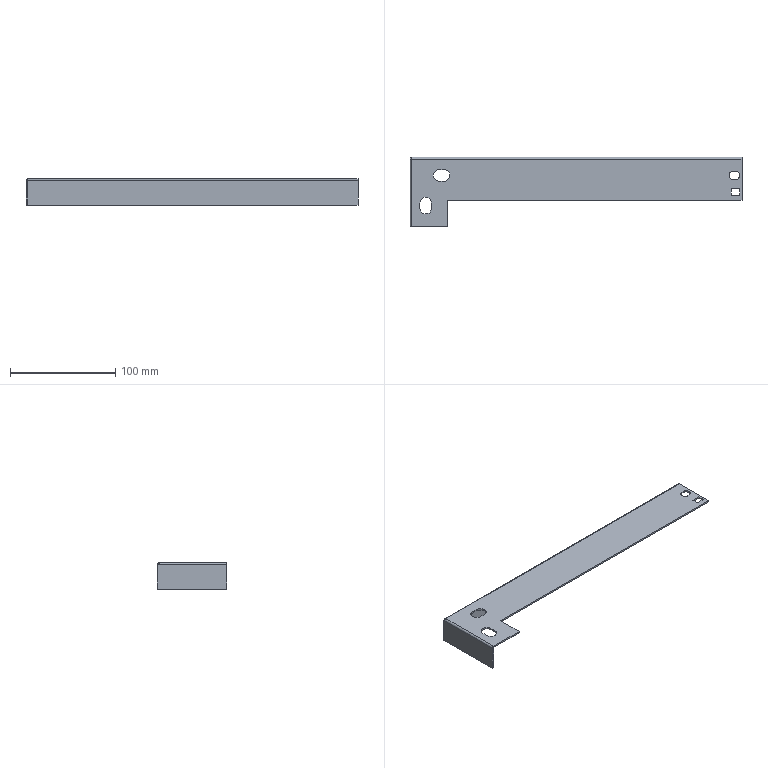Part | 1 solid | 43 faces | box 316 x 66 x 25 mm | volume 33332 mm3 | plane 31 | cylinder 12 | commonest cylinder face diameters 11 x5 8 x3 0.4 x2 3.4 x2
STEP:
#1=CARTESIAN_POINT('',(151.8,11.8,1.5));
#2=VERTEX_POINT('',#1);
#3=CARTESIAN_POINT('',(155.8,15.8,1.5));
#4=VERTEX_POINT('',#3);
#5=CARTESIAN_POINT('',(151.8,15.8,1.5));
#6=DIRECTION('',(0.,0.,1.));
#7=DIRECTION('',(1.,0.,0.));
#8=AXIS2_PLACEMENT_3D('',#5,#6,#7);
#9=CIRCLE('',#8,4.);
#10=EDGE_CURVE('',#2,#4,#9,.T.);
#11=ORIENTED_EDGE('',*,*,#10,.T.);
#12=CARTESIAN_POINT('',(155.8,15.8,0.));
#13=VERTEX_POINT('',#12);
#14=CARTESIAN_POINT('',(155.8,15.8,10.));
#15=DIRECTION('',(0.,0.,-1.));
#16=VECTOR('',#15,1000.);
#17=LINE('',#14,#16);
#18=EDGE_CURVE('',#4,#13,#17,.T.);
#19=ORIENTED_EDGE('',*,*,#18,.T.);
#20=CARTESIAN_POINT('',(151.8,11.8,0.));
#21=VERTEX_POINT('',#20);
#22=CARTESIAN_POINT('',(151.8,15.8,0.));
#23=DIRECTION('',(0.,0.,1.));
#24=DIRECTION('',(1.,0.,0.));
#25=AXIS2_PLACEMENT_3D('',#22,#23,#24);
#26=CIRCLE('',#25,4.);
#27=EDGE_CURVE('',#21,#13,#26,.T.);
#28=ORIENTED_EDGE('',*,*,#27,.F.);
#29=CARTESIAN_POINT('',(151.8,11.8,10.));
#30=DIRECTION('',(0.,0.,-1.));
#31=VECTOR('',#30,1000.);
#32=LINE('',#29,#31);
#33=EDGE_CURVE('',#2,#21,#32,.T.);
#34=ORIENTED_EDGE('',*,*,#33,.F.);
#35=EDGE_LOOP('',(#11,#19,#28,#34));
#36=FACE_OUTER_BOUND('',#35,.T.);
#37=CARTESIAN_POINT('',(151.8,15.8,10.));
#38=DIRECTION('',(0.,0.,-1.));
#39=DIRECTION('',(1.,0.,0.));
#40=AXIS2_PLACEMENT_3D('',#37,#38,#39);
#41=CYLINDRICAL_SURFACE('',#40,4.);
#42=ADVANCED_FACE('',(#36),#41,.F.);
#43=CARTESIAN_POINT('',(-125.5,10.3,1.5));
#44=VERTEX_POINT('',#43);
#45=CARTESIAN_POINT('',(-120.,15.8,1.5));
#46=VERTEX_POINT('',#45);
#47=CARTESIAN_POINT('',(-125.5,15.8,1.5));
#48=DIRECTION('',(0.,0.,1.));
#49=DIRECTION('',(1.,0.,0.));
#50=AXIS2_PLACEMENT_3D('',#47,#48,#49);
#51=CIRCLE('',#50,5.5);
#52=EDGE_CURVE('',#44,#46,#51,.T.);
#53=ORIENTED_EDGE('',*,*,#52,.T.);
#54=CARTESIAN_POINT('',(-120.,15.8,0.));
#55=VERTEX_POINT('',#54);
#56=CARTESIAN_POINT('',(-120.,15.8,10.));
#57=DIRECTION('',(0.,0.,-1.));
#58=VECTOR('',#57,1000.);
#59=LINE('',#56,#58);
#60=EDGE_CURVE('',#46,#55,#59,.T.);
#61=ORIENTED_EDGE('',*,*,#60,.T.);
#62=CARTESIAN_POINT('',(-125.5,10.3,0.));
#63=VERTEX_POINT('',#62);
#64=CARTESIAN_POINT('',(-125.5,15.8,0.));
#65=DIRECTION('',(0.,0.,1.));
#66=DIRECTION('',(1.,0.,0.));
#67=AXIS2_PLACEMENT_3D('',#64,#65,#66);
#68=CIRCLE('',#67,5.5);
#69=EDGE_CURVE('',#63,#55,#68,.T.);
#70=ORIENTED_EDGE('',*,*,#69,.F.);
#71=CARTESIAN_POINT('',(-125.5,10.3,10.));
#72=DIRECTION('',(0.,0.,-1.));
#73=VECTOR('',#72,1000.);
#74=LINE('',#71,#73);
#75=EDGE_CURVE('',#44,#63,#74,.T.);
#76=ORIENTED_EDGE('',*,*,#75,.F.);
#77=EDGE_LOOP('',(#53,#61,#70,#76));
#78=FACE_OUTER_BOUND('',#77,.T.);
#79=CARTESIAN_POINT('',(-125.5,15.8,10.));
#80=DIRECTION('',(0.,0.,-1.));
#81=DIRECTION('',(1.,0.,0.));
#82=AXIS2_PLACEMENT_3D('',#79,#80,#81);
#83=CYLINDRICAL_SURFACE('',#82,5.5);
#84=ADVANCED_FACE('',(#78),#83,.F.);
#85=CARTESIAN_POINT('',(158.,-8.,1.5));
#86=VERTEX_POINT('',#85);
#87=CARTESIAN_POINT('',(158.,31.3,1.5));
#88=VERTEX_POINT('',#87);
#89=CARTESIAN_POINT('',(158.,33.,1.5));
#90=DIRECTION('',(0.,1.,0.));
#91=VECTOR('',#90,1000.);
#92=LINE('',#89,#91);
#93=EDGE_CURVE('',#86,#88,#92,.T.);
#94=ORIENTED_EDGE('',*,*,#93,.T.);
#95=CARTESIAN_POINT('',(-156.3,31.3,1.5));
#96=VERTEX_POINT('',#95);
#97=CARTESIAN_POINT('',(-156.3,31.3,1.5));
#98=DIRECTION('',(1.,0.,0.));
#99=VECTOR('',#98,1000.);
#100=LINE('',#97,#99);
#101=EDGE_CURVE('',#96,#88,#100,.T.);
#102=ORIENTED_EDGE('',*,*,#101,.F.);
#103=CARTESIAN_POINT('',(-156.3,-33.,1.5));
#104=VERTEX_POINT('',#103);
#105=CARTESIAN_POINT('',(-156.3,-33.,1.5));
#106=DIRECTION('',(0.,1.,0.));
#107=VECTOR('',#106,1000.);
#108=LINE('',#105,#107);
#109=EDGE_CURVE('',#104,#96,#108,.T.);
#110=ORIENTED_EDGE('',*,*,#109,.F.);
#111=CARTESIAN_POINT('',(-122.,-33.,1.5));
#112=VERTEX_POINT('',#111);
#113=CARTESIAN_POINT('',(-158.,-33.,1.5));
#114=DIRECTION('',(1.,0.,0.));
#115=VECTOR('',#114,1000.);
#116=LINE('',#113,#115);
#117=EDGE_CURVE('',#104,#112,#116,.T.);
#118=ORIENTED_EDGE('',*,*,#117,.T.);
#119=CARTESIAN_POINT('',(-122.,-8.,1.5));
#120=VERTEX_POINT('',#119);
#121=CARTESIAN_POINT('',(-122.,0.,1.5));
#122=DIRECTION('',(0.,-1.,0.));
#123=VECTOR('',#122,1000.);
#124=LINE('',#121,#123);
#125=EDGE_CURVE('',#120,#112,#124,.T.);
#126=ORIENTED_EDGE('',*,*,#125,.F.);
#127=CARTESIAN_POINT('',(0.,-8.,1.5));
#128=DIRECTION('',(-1.,0.,0.));
#129=VECTOR('',#128,1000.);
#130=LINE('',#127,#129);
#131=EDGE_CURVE('',#86,#120,#130,.T.);
#132=ORIENTED_EDGE('',*,*,#131,.F.);
#133=EDGE_LOOP('',(#94,#102,#110,#118,#126,#132));
#134=FACE_OUTER_BOUND('',#133,.T.);
#135=CARTESIAN_POINT('',(-137.5,-15.5,1.5));
#136=VERTEX_POINT('',#135);
#137=CARTESIAN_POINT('',(-137.5,-10.5,1.5));
#138=VERTEX_POINT('',#137);
#139=CARTESIAN_POINT('',(-137.5,0.,1.5));
#140=DIRECTION('',(0.,1.,0.));
#141=VECTOR('',#140,1000.);
#142=LINE('',#139,#141);
#143=EDGE_CURVE('',#136,#138,#142,.T.);
#144=ORIENTED_EDGE('',*,*,#143,.F.);
#145=CARTESIAN_POINT('',(-148.5,-15.5,1.5));
#146=VERTEX_POINT('',#145);
#147=CARTESIAN_POINT('',(-143.,-15.5,1.5));
#148=DIRECTION('',(0.,0.,1.));
#149=DIRECTION('',(1.,0.,0.));
#150=AXIS2_PLACEMENT_3D('',#147,#148,#149);
#151=CIRCLE('',#150,5.5);
#152=EDGE_CURVE('',#146,#136,#151,.T.);
#153=ORIENTED_EDGE('',*,*,#152,.F.);
#154=CARTESIAN_POINT('',(-148.5,-10.5,1.5));
#155=VERTEX_POINT('',#154);
#156=CARTESIAN_POINT('',(-148.5,0.,1.5));
#157=DIRECTION('',(0.,-1.,0.));
#158=VECTOR('',#157,1000.);
#159=LINE('',#156,#158);
#160=EDGE_CURVE('',#155,#146,#159,.T.);
#161=ORIENTED_EDGE('',*,*,#160,.F.);
#162=CARTESIAN_POINT('',(-143.,-10.5,1.5));
#163=DIRECTION('',(0.,0.,1.));
#164=DIRECTION('',(1.,0.,0.));
#165=AXIS2_PLACEMENT_3D('',#162,#163,#164);
#166=CIRCLE('',#165,5.5);
#167=EDGE_CURVE('',#138,#155,#166,.T.);
#168=ORIENTED_EDGE('',*,*,#167,.F.);
#169=EDGE_LOOP('',(#144,#153,#161,#168));
#170=FACE_BOUND('',#169,.T.);
#171=CARTESIAN_POINT('',(-125.5,21.3,1.5));
#172=VERTEX_POINT('',#171);
#173=CARTESIAN_POINT('',(-130.5,21.3,1.5));
#174=VERTEX_POINT('',#173);
#175=CARTESIAN_POINT('',(0.,21.3,1.5));
#176=DIRECTION('',(-1.,0.,0.));
#177=VECTOR('',#176,1000.);
#178=LINE('',#175,#177);
#179=EDGE_CURVE('',#172,#174,#178,.T.);
#180=ORIENTED_EDGE('',*,*,#179,.F.);
#181=CARTESIAN_POINT('',(-125.5,15.8,1.5));
#182=DIRECTION('',(0.,0.,1.));
#183=DIRECTION('',(1.,0.,0.));
#184=AXIS2_PLACEMENT_3D('',#181,#182,#183);
#185=CIRCLE('',#184,5.5);
#186=EDGE_CURVE('',#46,#172,#185,.T.);
#187=ORIENTED_EDGE('',*,*,#186,.F.);
#188=ORIENTED_EDGE('',*,*,#52,.F.);
#189=CARTESIAN_POINT('',(-130.5,10.3,1.5));
#190=VERTEX_POINT('',#189);
#191=CARTESIAN_POINT('',(0.,10.3,1.5));
#192=DIRECTION('',(1.,0.,0.));
#193=VECTOR('',#192,1000.);
#194=LINE('',#191,#193);
#195=EDGE_CURVE('',#190,#44,#194,.T.);
#196=ORIENTED_EDGE('',*,*,#195,.F.);
#197=CARTESIAN_POINT('',(-130.5,15.8,1.5));
#198=DIRECTION('',(0.,0.,1.));
#199=DIRECTION('',(1.,0.,0.));
#200=AXIS2_PLACEMENT_3D('',#197,#198,#199);
#201=CIRCLE('',#200,5.5);
#202=EDGE_CURVE('',#174,#190,#201,.T.);
#203=ORIENTED_EDGE('',*,*,#202,.F.);
#204=EDGE_LOOP('',(#180,#187,#188,#196,#203));
#205=FACE_BOUND('',#204,.T.);
#206=CARTESIAN_POINT('',(151.8,19.8,1.5));
#207=VERTEX_POINT('',#206);
#208=CARTESIAN_POINT('',(149.8,19.8,1.5));
#209=VERTEX_POINT('',#208);
#210=CARTESIAN_POINT('',(0.,19.8,1.5));
#211=DIRECTION('',(-1.,0.,0.));
#212=VECTOR('',#211,1000.);
#213=LINE('',#210,#212);
#214=EDGE_CURVE('',#207,#209,#213,.T.);
#215=ORIENTED_EDGE('',*,*,#214,.F.);
#216=CARTESIAN_POINT('',(151.8,15.8,1.5));
#217=DIRECTION('',(0.,0.,1.));
#218=DIRECTION('',(1.,0.,0.));
#219=AXIS2_PLACEMENT_3D('',#216,#217,#218);
#220=CIRCLE('',#219,4.);
#221=EDGE_CURVE('',#4,#207,#220,.T.);
#222=ORIENTED_EDGE('',*,*,#221,.F.);
#223=ORIENTED_EDGE('',*,*,#10,.F.);
#224=CARTESIAN_POINT('',(149.8,11.8,1.5));
#225=VERTEX_POINT('',#224);
#226=CARTESIAN_POINT('',(0.,11.8,1.5));
#227=DIRECTION('',(1.,0.,0.));
#228=VECTOR('',#227,1000.);
#229=LINE('',#226,#228);
#230=EDGE_CURVE('',#225,#2,#229,.T.);
#231=ORIENTED_EDGE('',*,*,#230,.F.);
#232=CARTESIAN_POINT('',(149.8,15.8,1.5));
#233=DIRECTION('',(0.,0.,1.));
#234=DIRECTION('',(1.,0.,0.));
#235=AXIS2_PLACEMENT_3D('',#232,#233,#234);
#236=CIRCLE('',#235,4.);
#237=EDGE_CURVE('',#209,#225,#236,.T.);
#238=ORIENTED_EDGE('',*,*,#237,.F.);
#239=EDGE_LOOP('',(#215,#222,#223,#231,#238));
#240=FACE_BOUND('',#239,.T.);
#241=CARTESIAN_POINT('',(147.8,-3.,1.5));
#242=VERTEX_POINT('',#241);
#243=CARTESIAN_POINT('',(147.8,3.,1.5));
#244=VERTEX_POINT('',#243);
#245=CARTESIAN_POINT('',(147.8,0.,1.5));
#246=DIRECTION('',(0.,1.,0.));
#247=VECTOR('',#246,1000.);
#248=LINE('',#245,#247);
#249=EDGE_CURVE('',#242,#244,#248,.T.);
#250=ORIENTED_EDGE('',*,*,#249,.T.);
#251=CARTESIAN_POINT('',(155.8,3.,1.5));
#252=VERTEX_POINT('',#251);
#253=CARTESIAN_POINT('',(0.,3.,1.5));
#254=DIRECTION('',(1.,0.,0.));
#255=VECTOR('',#254,1000.);
#256=LINE('',#253,#255);
#257=EDGE_CURVE('',#244,#252,#256,.T.);
#258=ORIENTED_EDGE('',*,*,#257,.T.);
#259=CARTESIAN_POINT('',(155.8,-3.,1.5));
#260=VERTEX_POINT('',#259);
#261=CARTESIAN_POINT('',(155.8,0.,1.5));
#262=DIRECTION('',(0.,-1.,0.));
#263=VECTOR('',#262,1000.);
#264=LINE('',#261,#263);
#265=EDGE_CURVE('',#252,#260,#264,.T.);
#266=ORIENTED_EDGE('',*,*,#265,.T.);
#267=CARTESIAN_POINT('',(0.,-3.,1.5));
#268=DIRECTION('',(-1.,0.,0.));
#269=VECTOR('',#268,1000.);
#270=LINE('',#267,#269);
#271=EDGE_CURVE('',#260,#242,#270,.T.);
#272=ORIENTED_EDGE('',*,*,#271,.T.);
#273=EDGE_LOOP('',(#250,#258,#266,#272));
#274=FACE_BOUND('',#273,.T.);
#275=CARTESIAN_POINT('',(0.,0.,1.5));
#276=DIRECTION('',(0.,0.,-1.));
#277=DIRECTION('',(1.,0.,0.));
#278=AXIS2_PLACEMENT_3D('',#275,#276,#277);
#279=PLANE('',#278);
#280=ADVANCED_FACE('',(#134,#170,#205,#240,#274),#279,.F.);
#281=CARTESIAN_POINT('',(158.,-8.,0.));
#282=VERTEX_POINT('',#281);
#283=CARTESIAN_POINT('',(-122.,-8.,0.));
#284=VERTEX_POINT('',#283);
#285=CARTESIAN_POINT('',(0.,-8.,0.));
#286=DIRECTION('',(-1.,0.,0.));
#287=VECTOR('',#286,1000.);
#288=LINE('',#285,#287);
#289=EDGE_CURVE('',#282,#284,#288,.T.);
#290=ORIENTED_EDGE('',*,*,#289,.T.);
#291=CARTESIAN_POINT('',(-122.,-33.,0.));
#292=VERTEX_POINT('',#291);
#293=CARTESIAN_POINT('',(-122.,0.,0.));
#294=DIRECTION('',(0.,-1.,0.));
#295=VECTOR('',#294,1000.);
#296=LINE('',#293,#295);
#297=EDGE_CURVE('',#284,#292,#296,.T.);
#298=ORIENTED_EDGE('',*,*,#297,.T.);
#299=CARTESIAN_POINT('',(-156.3,-33.,0.));
#300=VERTEX_POINT('',#299);
#301=CARTESIAN_POINT('',(-158.,-33.,0.));
#302=DIRECTION('',(1.,0.,0.));
#303=VECTOR('',#302,1000.);
#304=LINE('',#301,#303);
#305=EDGE_CURVE('',#300,#292,#304,.T.);
#306=ORIENTED_EDGE('',*,*,#305,.F.);
#307=CARTESIAN_POINT('',(-156.3,31.3,0.));
#308=VERTEX_POINT('',#307);
#309=CARTESIAN_POINT('',(-156.3,-33.,0.));
#310=DIRECTION('',(0.,1.,0.));
#311=VECTOR('',#310,1000.);
#312=LINE('',#309,#311);
#313=EDGE_CURVE('',#300,#308,#312,.T.);
#314=ORIENTED_EDGE('',*,*,#313,.T.);
#315=CARTESIAN_POINT('',(158.,31.3,0.));
#316=VERTEX_POINT('',#315);
#317=CARTESIAN_POINT('',(-156.3,31.3,0.));
#318=DIRECTION('',(1.,0.,0.));
#319=VECTOR('',#318,1000.);
#320=LINE('',#317,#319);
#321=EDGE_CURVE('',#308,#316,#320,.T.);
#322=ORIENTED_EDGE('',*,*,#321,.T.);
#323=CARTESIAN_POINT('',(158.,33.,0.));
#324=DIRECTION('',(0.,1.,0.));
#325=VECTOR('',#324,1000.);
#326=LINE('',#323,#325);
#327=EDGE_CURVE('',#282,#316,#326,.T.);
#328=ORIENTED_EDGE('',*,*,#327,.F.);
#329=EDGE_LOOP('',(#290,#298,#306,#314,#322,#328));
#330=FACE_OUTER_BOUND('',#329,.T.);
#331=CARTESIAN_POINT('',(149.8,19.8,0.));
#332=VERTEX_POINT('',#331);
#333=CARTESIAN_POINT('',(149.8,11.8,0.));
#334=VERTEX_POINT('',#333);
#335=CARTESIAN_POINT('',(149.8,15.8,0.));
#336=DIRECTION('',(0.,0.,1.));
#337=DIRECTION('',(1.,0.,0.));
#338=AXIS2_PLACEMENT_3D('',#335,#336,#337);
#339=CIRCLE('',#338,4.);
#340=EDGE_CURVE('',#332,#334,#339,.T.);
#341=ORIENTED_EDGE('',*,*,#340,.T.);
#342=CARTESIAN_POINT('',(149.8,11.8,0.));
#343=DIRECTION('',(1.,0.,0.));
#344=VECTOR('',#343,1000.);
#345=LINE('',#342,#344);
#346=EDGE_CURVE('',#334,#21,#345,.T.);
#347=ORIENTED_EDGE('',*,*,#346,.T.);
#348=ORIENTED_EDGE('',*,*,#27,.T.);
#349=CARTESIAN_POINT('',(151.8,19.8,0.));
#350=VERTEX_POINT('',#349);
#351=CARTESIAN_POINT('',(151.8,15.8,0.));
#352=DIRECTION('',(0.,0.,1.));
#353=DIRECTION('',(1.,0.,0.));
#354=AXIS2_PLACEMENT_3D('',#351,#352,#353);
#355=CIRCLE('',#354,4.);
#356=EDGE_CURVE('',#13,#350,#355,.T.);
#357=ORIENTED_EDGE('',*,*,#356,.T.);
#358=CARTESIAN_POINT('',(149.8,19.8,0.));
#359=DIRECTION('',(-1.,0.,0.));
#360=VECTOR('',#359,1000.);
#361=LINE('',#358,#360);
#362=EDGE_CURVE('',#350,#332,#361,.T.);
#363=ORIENTED_EDGE('',*,*,#362,.T.);
#364=EDGE_LOOP('',(#341,#347,#348,#357,#363));
#365=FACE_BOUND('',#364,.T.);
#366=CARTESIAN_POINT('',(-130.5,21.3,0.));
#367=VERTEX_POINT('',#366);
#368=CARTESIAN_POINT('',(-130.5,10.3,0.));
#369=VERTEX_POINT('',#368);
#370=CARTESIAN_POINT('',(-130.5,15.8,0.));
#371=DIRECTION('',(0.,0.,1.));
#372=DIRECTION('',(1.,0.,0.));
#373=AXIS2_PLACEMENT_3D('',#370,#371,#372);
#374=CIRCLE('',#373,5.5);
#375=EDGE_CURVE('',#367,#369,#374,.T.);
#376=ORIENTED_EDGE('',*,*,#375,.T.);
#377=CARTESIAN_POINT('',(-130.5,10.3,0.));
#378=DIRECTION('',(1.,0.,0.));
#379=VECTOR('',#378,1000.);
#380=LINE('',#377,#379);
#381=EDGE_CURVE('',#369,#63,#380,.T.);
#382=ORIENTED_EDGE('',*,*,#381,.T.);
#383=ORIENTED_EDGE('',*,*,#69,.T.);
#384=CARTESIAN_POINT('',(-125.5,21.3,0.));
#385=VERTEX_POINT('',#384);
#386=CARTESIAN_POINT('',(-125.5,15.8,0.));
#387=DIRECTION('',(0.,0.,1.));
#388=DIRECTION('',(1.,0.,0.));
#389=AXIS2_PLACEMENT_3D('',#386,#387,#388);
#390=CIRCLE('',#389,5.5);
#391=EDGE_CURVE('',#55,#385,#390,.T.);
#392=ORIENTED_EDGE('',*,*,#391,.T.);
#393=CARTESIAN_POINT('',(-130.5,21.3,0.));
#394=DIRECTION('',(-1.,0.,0.));
#395=VECTOR('',#394,1000.);
#396=LINE('',#393,#395);
#397=EDGE_CURVE('',#385,#367,#396,.T.);
#398=ORIENTED_EDGE('',*,*,#397,.T.);
#399=EDGE_LOOP('',(#376,#382,#383,#392,#398));
#400=FACE_BOUND('',#399,.T.);
#401=CARTESIAN_POINT('',(-137.5,-10.5,0.));
#402=VERTEX_POINT('',#401);
#403=CARTESIAN_POINT('',(-148.5,-10.5,0.));
#404=VERTEX_POINT('',#403);
#405=CARTESIAN_POINT('',(-143.,-10.5,0.));
#406=DIRECTION('',(0.,0.,1.));
#407=DIRECTION('',(1.,0.,0.));
#408=AXIS2_PLACEMENT_3D('',#405,#406,#407);
#409=CIRCLE('',#408,5.5);
#410=EDGE_CURVE('',#402,#404,#409,.T.);
#411=ORIENTED_EDGE('',*,*,#410,.T.);
#412=CARTESIAN_POINT('',(-148.5,-15.5,0.));
#413=VERTEX_POINT('',#412);
#414=CARTESIAN_POINT('',(-148.5,-10.5,0.));
#415=DIRECTION('',(0.,-1.,0.));
#416=VECTOR('',#415,1000.);
#417=LINE('',#414,#416);
#418=EDGE_CURVE('',#404,#413,#417,.T.);
#419=ORIENTED_EDGE('',*,*,#418,.T.);
#420=CARTESIAN_POINT('',(-137.5,-15.5,0.));
#421=VERTEX_POINT('',#420);
#422=CARTESIAN_POINT('',(-143.,-15.5,0.));
#423=DIRECTION('',(0.,0.,1.));
#424=DIRECTION('',(1.,0.,0.));
#425=AXIS2_PLACEMENT_3D('',#422,#423,#424);
#426=CIRCLE('',#425,5.5);
#427=EDGE_CURVE('',#413,#421,#426,.T.);
#428=ORIENTED_EDGE('',*,*,#427,.T.);
#429=CARTESIAN_POINT('',(-137.5,-10.5,0.));
#430=DIRECTION('',(0.,1.,0.));
#431=VECTOR('',#430,1000.);
#432=LINE('',#429,#431);
#433=EDGE_CURVE('',#421,#402,#432,.T.);
#434=ORIENTED_EDGE('',*,*,#433,.T.);
#435=EDGE_LOOP('',(#411,#419,#428,#434));
#436=FACE_BOUND('',#435,.T.);
#437=CARTESIAN_POINT('',(155.8,-3.,0.));
#438=VERTEX_POINT('',#437);
#439=CARTESIAN_POINT('',(147.8,-3.,0.));
#440=VERTEX_POINT('',#439);
#441=CARTESIAN_POINT('',(0.,-3.,0.));
#442=DIRECTION('',(-1.,0.,0.));
#443=VECTOR('',#442,1000.);
#444=LINE('',#441,#443);
#445=EDGE_CURVE('',#438,#440,#444,.T.);
#446=ORIENTED_EDGE('',*,*,#445,.F.);
#447=CARTESIAN_POINT('',(155.8,3.,0.));
#448=VERTEX_POINT('',#447);
#449=CARTESIAN_POINT('',(155.8,0.,0.));
#450=DIRECTION('',(0.,-1.,0.));
#451=VECTOR('',#450,1000.);
#452=LINE('',#449,#451);
#453=EDGE_CURVE('',#448,#438,#452,.T.);
#454=ORIENTED_EDGE('',*,*,#453,.F.);
#455=CARTESIAN_POINT('',(147.8,3.,0.));
#456=VERTEX_POINT('',#455);
#457=CARTESIAN_POINT('',(0.,3.,0.));
#458=DIRECTION('',(1.,0.,0.));
#459=VECTOR('',#458,1000.);
#460=LINE('',#457,#459);
#461=EDGE_CURVE('',#456,#448,#460,.T.);
#462=ORIENTED_EDGE('',*,*,#461,.F.);
#463=CARTESIAN_POINT('',(147.8,0.,0.));
#464=DIRECTION('',(0.,1.,0.));
#465=VECTOR('',#464,1000.);
#466=LINE('',#463,#465);
#467=EDGE_CURVE('',#440,#456,#466,.T.);
#468=ORIENTED_EDGE('',*,*,#467,.F.);
#469=EDGE_LOOP('',(#446,#454,#462,#468));
#470=FACE_BOUND('',#469,.T.);
#471=CARTESIAN_POINT('',(0.,0.,0.));
#472=DIRECTION('',(0.,0.,-1.));
#473=DIRECTION('',(1.,0.,0.));
#474=AXIS2_PLACEMENT_3D('',#471,#472,#473);
#475=PLANE('',#474);
#476=ADVANCED_FACE('',(#330,#365,#400,#436,#470),#475,.T.);
#477=CARTESIAN_POINT('',(-158.,31.3,-0.2));
#478=VERTEX_POINT('',#477);
#479=CARTESIAN_POINT('',(-156.5,31.3,-0.2));
#480=VERTEX_POINT('',#479);
#481=CARTESIAN_POINT('',(-158.,31.3,-0.2));
#482=DIRECTION('',(1.,0.,0.));
#483=VECTOR('',#482,1000.);
#484=LINE('',#481,#483);
#485=EDGE_CURVE('',#478,#480,#484,.T.);
#486=ORIENTED_EDGE('',*,*,#485,.T.);
#487=CARTESIAN_POINT('',(-156.5,33.,-0.2));
#488=VERTEX_POINT('',#487);
#489=CARTESIAN_POINT('',(-156.5,33.,-0.2));
#490=DIRECTION('',(0.,-1.,0.));
#491=VECTOR('',#490,1000.);
#492=LINE('',#489,#491);
#493=EDGE_CURVE('',#488,#480,#492,.T.);
#494=ORIENTED_EDGE('',*,*,#493,.F.);
#495=CARTESIAN_POINT('',(-158.,33.,-0.2));
#496=VERTEX_POINT('',#495);
#497=CARTESIAN_POINT('',(-158.,33.,-0.2));
#498=DIRECTION('',(-1.,0.,0.));
#499=VECTOR('',#498,1000.);
#500=LINE('',#497,#499);
#501=EDGE_CURVE('',#488,#496,#500,.T.);
#502=ORIENTED_EDGE('',*,*,#501,.T.);
#503=CARTESIAN_POINT('',(-158.,33.,-0.2));
#504=DIRECTION('',(0.,1.,0.));
#505=VECTOR('',#504,1000.);
#506=LINE('',#503,#505);
#507=EDGE_CURVE('',#478,#496,#506,.T.);
#508=ORIENTED_EDGE('',*,*,#507,.F.);
#509=EDGE_LOOP('',(#486,#494,#502,#508));
#510=FACE_OUTER_BOUND('',#509,.T.);
#511=CARTESIAN_POINT('',(0.,0.,-0.2));
#512=DIRECTION('',(0.,0.,1.));
#513=DIRECTION('',(-1.,0.,0.));
#514=AXIS2_PLACEMENT_3D('',#511,#512,#513);
#515=PLANE('',#514);
#516=ADVANCED_FACE('',(#510),#515,.T.);
#517=CARTESIAN_POINT('',(-158.,-33.,-0.2));
#518=VERTEX_POINT('',#517);
#519=CARTESIAN_POINT('',(-158.,33.,-0.2));
#520=DIRECTION('',(0.,1.,0.));
#521=VECTOR('',#520,1000.);
#522=LINE('',#519,#521);
#523=EDGE_CURVE('',#518,#478,#522,.T.);
#524=ORIENTED_EDGE('',*,*,#523,.F.);
#525=CARTESIAN_POINT('',(-156.3,-33.,-0.2));
#526=DIRECTION('',(0.,1.,0.));
#527=DIRECTION('',(0.,0.,1.));
#528=AXIS2_PLACEMENT_3D('',#525,#526,#527);
#529=CIRCLE('',#528,1.7);
#530=EDGE_CURVE('',#518,#104,#529,.T.);
#531=ORIENTED_EDGE('',*,*,#530,.T.);
#532=ORIENTED_EDGE('',*,*,#109,.T.);
#533=CARTESIAN_POINT('',(-156.3,31.3,-0.2));
#534=DIRECTION('',(0.,1.,0.));
#535=DIRECTION('',(0.,0.,-1.));
#536=AXIS2_PLACEMENT_3D('',#533,#534,#535);
#537=CIRCLE('',#536,1.7);
#538=EDGE_CURVE('',#478,#96,#537,.T.);
#539=ORIENTED_EDGE('',*,*,#538,.F.);
#540=EDGE_LOOP('',(#524,#531,#532,#539));
#541=FACE_OUTER_BOUND('',#540,.T.);
#542=CARTESIAN_POINT('',(-156.3,-33.,-0.2));
#543=DIRECTION('',(0.,-1.,0.));
#544=DIRECTION('',(-1.,0.,0.));
#545=AXIS2_PLACEMENT_3D('',#542,#543,#544);
#546=CYLINDRICAL_SURFACE('',#545,1.7);
#547=ADVANCED_FACE('',(#541),#546,.T.);
#548=CARTESIAN_POINT('',(-122.,-33.,-23.5));
#549=DIRECTION('',(0.,0.,1.));
#550=VECTOR('',#549,1000.);
#551=LINE('',#548,#550);
#552=EDGE_CURVE('',#292,#112,#551,.T.);
#553=ORIENTED_EDGE('',*,*,#552,.T.);
#554=ORIENTED_EDGE('',*,*,#117,.F.);
#555=CARTESIAN_POINT('',(-156.3,-33.,0.));
#556=DIRECTION('',(0.,0.,1.));
#557=VECTOR('',#556,1000.);
#558=LINE('',#555,#557);
#559=EDGE_CURVE('',#300,#104,#558,.T.);
#560=ORIENTED_EDGE('',*,*,#559,.F.);
#561=ORIENTED_EDGE('',*,*,#305,.T.);
#562=EDGE_LOOP('',(#553,#554,#560,#561));
#563=FACE_OUTER_BOUND('',#562,.T.);
#564=CARTESIAN_POINT('',(-158.,-33.,1.5));
#565=DIRECTION('',(0.,-1.,0.));
#566=DIRECTION('',(0.,0.,1.));
#567=AXIS2_PLACEMENT_3D('',#564,#565,#566);
#568=PLANE('',#567);
#569=ADVANCED_FACE('',(#563),#568,.T.);
#570=CARTESIAN_POINT('',(158.,-8.,1.5));
#571=DIRECTION('',(0.,0.,-1.));
#572=VECTOR('',#571,1000.);
#573=LINE('',#570,#572);
#574=EDGE_CURVE('',#86,#282,#573,.T.);
#575=ORIENTED_EDGE('',*,*,#574,.T.);
#576=ORIENTED_EDGE('',*,*,#327,.T.);
#577=CARTESIAN_POINT('',(158.,31.3,0.));
#578=DIRECTION('',(0.,0.,1.));
#579=VECTOR('',#578,1000.);
#580=LINE('',#577,#579);
#581=EDGE_CURVE('',#316,#88,#580,.T.);
#582=ORIENTED_EDGE('',*,*,#581,.T.);
#583=ORIENTED_EDGE('',*,*,#93,.F.);
#584=EDGE_LOOP('',(#575,#576,#582,#583));
#585=FACE_OUTER_BOUND('',#584,.T.);
#586=CARTESIAN_POINT('',(158.,33.,1.5));
#587=DIRECTION('',(1.,0.,0.));
#588=DIRECTION('',(0.,1.,0.));
#589=AXIS2_PLACEMENT_3D('',#586,#587,#588);
#590=PLANE('',#589);
#591=ADVANCED_FACE('',(#585),#590,.T.);
#592=CARTESIAN_POINT('',(-137.5,-10.5,10.));
#593=DIRECTION('',(0.,0.,-1.));
#594=VECTOR('',#593,1000.);
#595=LINE('',#592,#594);
#596=EDGE_CURVE('',#138,#402,#595,.T.);
#597=ORIENTED_EDGE('',*,*,#596,.F.);
#598=ORIENTED_EDGE('',*,*,#167,.T.);
#599=CARTESIAN_POINT('',(-148.5,-10.5,10.));
#600=DIRECTION('',(0.,0.,-1.));
#601=VECTOR('',#600,1000.);
#602=LINE('',#599,#601);
#603=EDGE_CURVE('',#155,#404,#602,.T.);
#604=ORIENTED_EDGE('',*,*,#603,.T.);
#605=ORIENTED_EDGE('',*,*,#410,.F.);
#606=EDGE_LOOP('',(#597,#598,#604,#605));
#607=FACE_OUTER_BOUND('',#606,.T.);
#608=CARTESIAN_POINT('',(-143.,-10.5,10.));
#609=DIRECTION('',(0.,0.,-1.));
#610=DIRECTION('',(1.,0.,0.));
#611=AXIS2_PLACEMENT_3D('',#608,#609,#610);
#612=CYLINDRICAL_SURFACE('',#611,5.5);
#613=ADVANCED_FACE('',(#607),#612,.F.);
#614=CARTESIAN_POINT('',(-137.5,-15.5,10.));
#615=DIRECTION('',(0.,0.,-1.));
#616=VECTOR('',#615,1000.);
#617=LINE('',#614,#616);
#618=EDGE_CURVE('',#136,#421,#617,.T.);
#619=ORIENTED_EDGE('',*,*,#618,.F.);
#620=ORIENTED_EDGE('',*,*,#143,.T.);
#621=ORIENTED_EDGE('',*,*,#596,.T.);
#622=ORIENTED_EDGE('',*,*,#433,.F.);
#623=EDGE_LOOP('',(#619,#620,#621,#622));
#624=FACE_OUTER_BOUND('',#623,.T.);
#625=CARTESIAN_POINT('',(-137.5,-10.5,10.));
#626=DIRECTION('',(1.,0.,0.));
#627=DIRECTION('',(0.,0.,1.));
#628=AXIS2_PLACEMENT_3D('',#625,#626,#627);
#629=PLANE('',#628);
#630=ADVANCED_FACE('',(#624),#629,.F.);
#631=CARTESIAN_POINT('',(-148.5,-15.5,10.));
#632=DIRECTION('',(0.,0.,-1.));
#633=VECTOR('',#632,1000.);
#634=LINE('',#631,#633);
#635=EDGE_CURVE('',#146,#413,#634,.T.);
#636=ORIENTED_EDGE('',*,*,#635,.F.);
#637=ORIENTED_EDGE('',*,*,#152,.T.);
#638=ORIENTED_EDGE('',*,*,#618,.T.);
#639=ORIENTED_EDGE('',*,*,#427,.F.);
#640=EDGE_LOOP('',(#636,#637,#638,#639));
#641=FACE_OUTER_BOUND('',#640,.T.);
#642=CARTESIAN_POINT('',(-143.,-15.5,10.));
#643=DIRECTION('',(0.,0.,-1.));
#644=DIRECTION('',(1.,0.,0.));
#645=AXIS2_PLACEMENT_3D('',#642,#643,#644);
#646=CYLINDRICAL_SURFACE('',#645,5.5);
#647=ADVANCED_FACE('',(#641),#646,.F.);
#648=ORIENTED_EDGE('',*,*,#603,.F.);
#649=ORIENTED_EDGE('',*,*,#160,.T.);
#650=ORIENTED_EDGE('',*,*,#635,.T.);
#651=ORIENTED_EDGE('',*,*,#418,.F.);
#652=EDGE_LOOP('',(#648,#649,#650,#651));
#653=FACE_OUTER_BOUND('',#652,.T.);
#654=CARTESIAN_POINT('',(-148.5,-10.5,10.));
#655=DIRECTION('',(-1.,0.,0.));
#656=DIRECTION('',(0.,0.,-1.));
#657=AXIS2_PLACEMENT_3D('',#654,#655,#656);
#658=PLANE('',#657);
#659=ADVANCED_FACE('',(#653),#658,.F.);
#660=CARTESIAN_POINT('',(-130.5,21.3,10.));
#661=DIRECTION('',(0.,0.,-1.));
#662=VECTOR('',#661,1000.);
#663=LINE('',#660,#662);
#664=EDGE_CURVE('',#174,#367,#663,.T.);
#665=ORIENTED_EDGE('',*,*,#664,.F.);
#666=ORIENTED_EDGE('',*,*,#202,.T.);
#667=CARTESIAN_POINT('',(-130.5,10.3,10.));
#668=DIRECTION('',(0.,0.,-1.));
#669=VECTOR('',#668,1000.);
#670=LINE('',#667,#669);
#671=EDGE_CURVE('',#190,#369,#670,.T.);
#672=ORIENTED_EDGE('',*,*,#671,.T.);
#673=ORIENTED_EDGE('',*,*,#375,.F.);
#674=EDGE_LOOP('',(#665,#666,#672,#673));
#675=FACE_OUTER_BOUND('',#674,.T.);
#676=CARTESIAN_POINT('',(-130.5,15.8,10.));
#677=DIRECTION('',(0.,0.,-1.));
#678=DIRECTION('',(1.,0.,0.));
#679=AXIS2_PLACEMENT_3D('',#676,#677,#678);
#680=CYLINDRICAL_SURFACE('',#679,5.5);
#681=ADVANCED_FACE('',(#675),#680,.F.);
#682=CARTESIAN_POINT('',(-125.5,21.3,10.));
#683=DIRECTION('',(0.,0.,-1.));
#684=VECTOR('',#683,1000.);
#685=LINE('',#682,#684);
#686=EDGE_CURVE('',#172,#385,#685,.T.);
#687=ORIENTED_EDGE('',*,*,#686,.F.);
#688=ORIENTED_EDGE('',*,*,#179,.T.);
#689=ORIENTED_EDGE('',*,*,#664,.T.);
#690=ORIENTED_EDGE('',*,*,#397,.F.);
#691=EDGE_LOOP('',(#687,#688,#689,#690));
#692=FACE_OUTER_BOUND('',#691,.T.);
#693=CARTESIAN_POINT('',(-130.5,21.3,10.));
#694=DIRECTION('',(0.,1.,0.));
#695=DIRECTION('',(0.,0.,-1.));
#696=AXIS2_PLACEMENT_3D('',#693,#694,#695);
#697=PLANE('',#696);
#698=ADVANCED_FACE('',(#692),#697,.F.);
#699=ORIENTED_EDGE('',*,*,#60,.F.);
#700=ORIENTED_EDGE('',*,*,#186,.T.);
#701=ORIENTED_EDGE('',*,*,#686,.T.);
#702=ORIENTED_EDGE('',*,*,#391,.F.);
#703=EDGE_LOOP('',(#699,#700,#701,#702));
#704=FACE_OUTER_BOUND('',#703,.T.);
#705=CARTESIAN_POINT('',(-125.5,15.8,10.));
#706=DIRECTION('',(0.,0.,-1.));
#707=DIRECTION('',(1.,0.,0.));
#708=AXIS2_PLACEMENT_3D('',#705,#706,#707);
#709=CYLINDRICAL_SURFACE('',#708,5.5);
#710=ADVANCED_FACE('',(#704),#709,.F.);
#711=ORIENTED_EDGE('',*,*,#671,.F.);
#712=ORIENTED_EDGE('',*,*,#195,.T.);
#713=ORIENTED_EDGE('',*,*,#75,.T.);
#714=ORIENTED_EDGE('',*,*,#381,.F.);
#715=EDGE_LOOP('',(#711,#712,#713,#714));
#716=FACE_OUTER_BOUND('',#715,.T.);
#717=CARTESIAN_POINT('',(-130.5,10.3,10.));
#718=DIRECTION('',(0.,-1.,0.));
#719=DIRECTION('',(1.,0.,0.));
#720=AXIS2_PLACEMENT_3D('',#717,#718,#719);
#721=PLANE('',#720);
#722=ADVANCED_FACE('',(#716),#721,.F.);
#723=CARTESIAN_POINT('',(149.8,19.8,10.));
#724=DIRECTION('',(0.,0.,-1.));
#725=VECTOR('',#724,1000.);
#726=LINE('',#723,#725);
#727=EDGE_CURVE('',#209,#332,#726,.T.);
#728=ORIENTED_EDGE('',*,*,#727,.F.);
#729=ORIENTED_EDGE('',*,*,#237,.T.);
#730=CARTESIAN_POINT('',(149.8,11.8,10.));
#731=DIRECTION('',(0.,0.,-1.));
#732=VECTOR('',#731,1000.);
#733=LINE('',#730,#732);
#734=EDGE_CURVE('',#225,#334,#733,.T.);
#735=ORIENTED_EDGE('',*,*,#734,.T.);
#736=ORIENTED_EDGE('',*,*,#340,.F.);
#737=EDGE_LOOP('',(#728,#729,#735,#736));
#738=FACE_OUTER_BOUND('',#737,.T.);
#739=CARTESIAN_POINT('',(149.8,15.8,10.));
#740=DIRECTION('',(0.,0.,-1.));
#741=DIRECTION('',(1.,0.,0.));
#742=AXIS2_PLACEMENT_3D('',#739,#740,#741);
#743=CYLINDRICAL_SURFACE('',#742,4.);
#744=ADVANCED_FACE('',(#738),#743,.F.);
#745=CARTESIAN_POINT('',(151.8,19.8,10.));
#746=DIRECTION('',(0.,0.,-1.));
#747=VECTOR('',#746,1000.);
#748=LINE('',#745,#747);
#749=EDGE_CURVE('',#207,#350,#748,.T.);
#750=ORIENTED_EDGE('',*,*,#749,.F.);
#751=ORIENTED_EDGE('',*,*,#214,.T.);
#752=ORIENTED_EDGE('',*,*,#727,.T.);
#753=ORIENTED_EDGE('',*,*,#362,.F.);
#754=EDGE_LOOP('',(#750,#751,#752,#753));
#755=FACE_OUTER_BOUND('',#754,.T.);
#756=CARTESIAN_POINT('',(149.8,19.8,10.));
#757=DIRECTION('',(0.,1.,0.));
#758=DIRECTION('',(0.,0.,-1.));
#759=AXIS2_PLACEMENT_3D('',#756,#757,#758);
#760=PLANE('',#759);
#761=ADVANCED_FACE('',(#755),#760,.F.);
#762=ORIENTED_EDGE('',*,*,#18,.F.);
#763=ORIENTED_EDGE('',*,*,#221,.T.);
#764=ORIENTED_EDGE('',*,*,#749,.T.);
#765=ORIENTED_EDGE('',*,*,#356,.F.);
#766=EDGE_LOOP('',(#762,#763,#764,#765));
#767=FACE_OUTER_BOUND('',#766,.T.);
#768=CARTESIAN_POINT('',(151.8,15.8,10.));
#769=DIRECTION('',(0.,0.,-1.));
#770=DIRECTION('',(1.,0.,0.));
#771=AXIS2_PLACEMENT_3D('',#768,#769,#770);
#772=CYLINDRICAL_SURFACE('',#771,4.);
#773=ADVANCED_FACE('',(#767),#772,.F.);
#774=ORIENTED_EDGE('',*,*,#734,.F.);
#775=ORIENTED_EDGE('',*,*,#230,.T.);
#776=ORIENTED_EDGE('',*,*,#33,.T.);
#777=ORIENTED_EDGE('',*,*,#346,.F.);
#778=EDGE_LOOP('',(#774,#775,#776,#777));
#779=FACE_OUTER_BOUND('',#778,.T.);
#780=CARTESIAN_POINT('',(149.8,11.8,10.));
#781=DIRECTION('',(0.,-1.,0.));
#782=DIRECTION('',(0.,0.,1.));
#783=AXIS2_PLACEMENT_3D('',#780,#781,#782);
#784=PLANE('',#783);
#785=ADVANCED_FACE('',(#779),#784,.F.);
#786=CARTESIAN_POINT('',(-156.5,-33.,-0.2));
#787=VERTEX_POINT('',#786);
#788=CARTESIAN_POINT('',(-156.3,-33.,-0.2));
#789=DIRECTION('',(0.,1.,0.));
#790=DIRECTION('',(0.,0.,1.));
#791=AXIS2_PLACEMENT_3D('',#788,#789,#790);
#792=CIRCLE('',#791,0.2);
#793=EDGE_CURVE('',#787,#300,#792,.T.);
#794=ORIENTED_EDGE('',*,*,#793,.T.);
#795=ORIENTED_EDGE('',*,*,#559,.T.);
#796=ORIENTED_EDGE('',*,*,#530,.F.);
#797=CARTESIAN_POINT('',(-156.5,-33.,-0.2));
#798=DIRECTION('',(-1.,0.,0.));
#799=VECTOR('',#798,1000.);
#800=LINE('',#797,#799);
#801=EDGE_CURVE('',#787,#518,#800,.T.);
#802=ORIENTED_EDGE('',*,*,#801,.F.);
#803=EDGE_LOOP('',(#794,#795,#796,#802));
#804=FACE_OUTER_BOUND('',#803,.T.);
#805=CARTESIAN_POINT('',(-156.3,-33.,-0.2));
#806=DIRECTION('',(0.,1.,0.));
#807=DIRECTION('',(0.,0.,-1.));
#808=AXIS2_PLACEMENT_3D('',#805,#806,#807);
#809=PLANE('',#808);
#810=ADVANCED_FACE('',(#804),#809,.F.);
#811=ORIENTED_EDGE('',*,*,#538,.T.);
#812=CARTESIAN_POINT('',(-156.3,31.3,0.));
#813=DIRECTION('',(0.,0.,1.));
#814=VECTOR('',#813,1000.);
#815=LINE('',#812,#814);
#816=EDGE_CURVE('',#308,#96,#815,.T.);
#817=ORIENTED_EDGE('',*,*,#816,.F.);
#818=CARTESIAN_POINT('',(-156.3,31.3,-0.2));
#819=DIRECTION('',(0.,1.,0.));
#820=DIRECTION('',(0.,0.,-1.));
#821=AXIS2_PLACEMENT_3D('',#818,#819,#820);
#822=CIRCLE('',#821,0.2);
#823=EDGE_CURVE('',#480,#308,#822,.T.);
#824=ORIENTED_EDGE('',*,*,#823,.F.);
#825=ORIENTED_EDGE('',*,*,#485,.F.);
#826=EDGE_LOOP('',(#811,#817,#824,#825));
#827=FACE_OUTER_BOUND('',#826,.T.);
#828=CARTESIAN_POINT('',(-156.3,31.3,-0.2));
#829=DIRECTION('',(0.,1.,0.));
#830=DIRECTION('',(0.,0.,-1.));
#831=AXIS2_PLACEMENT_3D('',#828,#829,#830);
#832=PLANE('',#831);
#833=ADVANCED_FACE('',(#827),#832,.T.);
#834=ORIENTED_EDGE('',*,*,#823,.T.);
#835=ORIENTED_EDGE('',*,*,#313,.F.);
#836=ORIENTED_EDGE('',*,*,#793,.F.);
#837=CARTESIAN_POINT('',(-156.5,33.,-0.2));
#838=DIRECTION('',(0.,-1.,0.));
#839=VECTOR('',#838,1000.);
#840=LINE('',#837,#839);
#841=EDGE_CURVE('',#480,#787,#840,.T.);
#842=ORIENTED_EDGE('',*,*,#841,.F.);
#843=EDGE_LOOP('',(#834,#835,#836,#842));
#844=FACE_OUTER_BOUND('',#843,.T.);
#845=CARTESIAN_POINT('',(-156.3,-33.,-0.2));
#846=DIRECTION('',(0.,-1.,0.));
#847=DIRECTION('',(-1.,0.,0.));
#848=AXIS2_PLACEMENT_3D('',#845,#846,#847);
#849=CYLINDRICAL_SURFACE('',#848,0.2);
#850=ADVANCED_FACE('',(#844),#849,.F.);
#851=ORIENTED_EDGE('',*,*,#501,.F.);
#852=CARTESIAN_POINT('',(-156.5,33.,-23.5));
#853=VERTEX_POINT('',#852);
#854=CARTESIAN_POINT('',(-156.5,33.,0.));
#855=DIRECTION('',(0.,0.,1.));
#856=VECTOR('',#855,1000.);
#857=LINE('',#854,#856);
#858=EDGE_CURVE('',#853,#488,#857,.T.);
#859=ORIENTED_EDGE('',*,*,#858,.F.);
#860=CARTESIAN_POINT('',(-158.,33.,-23.5));
#861=VERTEX_POINT('',#860);
#862=CARTESIAN_POINT('',(-158.,33.,-23.5));
#863=DIRECTION('',(1.,0.,0.));
#864=VECTOR('',#863,1000.);
#865=LINE('',#862,#864);
#866=EDGE_CURVE('',#861,#853,#865,.T.);
#867=ORIENTED_EDGE('',*,*,#866,.F.);
#868=CARTESIAN_POINT('',(-158.,33.,0.));
#869=DIRECTION('',(0.,0.,1.));
#870=VECTOR('',#869,1000.);
#871=LINE('',#868,#870);
#872=EDGE_CURVE('',#861,#496,#871,.T.);
#873=ORIENTED_EDGE('',*,*,#872,.T.);
#874=EDGE_LOOP('',(#851,#859,#867,#873));
#875=FACE_OUTER_BOUND('',#874,.T.);
#876=CARTESIAN_POINT('',(-158.,33.,0.));
#877=DIRECTION('',(0.,-1.,0.));
#878=DIRECTION('',(0.,0.,1.));
#879=AXIS2_PLACEMENT_3D('',#876,#877,#878);
#880=PLANE('',#879);
#881=ADVANCED_FACE('',(#875),#880,.F.);
#882=ORIENTED_EDGE('',*,*,#801,.T.);
#883=CARTESIAN_POINT('',(-158.,-33.,-23.5));
#884=VERTEX_POINT('',#883);
#885=CARTESIAN_POINT('',(-158.,-33.,0.));
#886=DIRECTION('',(0.,0.,-1.));
#887=VECTOR('',#886,1000.);
#888=LINE('',#885,#887);
#889=EDGE_CURVE('',#518,#884,#888,.T.);
#890=ORIENTED_EDGE('',*,*,#889,.T.);
#891=CARTESIAN_POINT('',(-156.5,-33.,-23.5));
#892=VERTEX_POINT('',#891);
#893=CARTESIAN_POINT('',(-158.,-33.,-23.5));
#894=DIRECTION('',(1.,0.,0.));
#895=VECTOR('',#894,1000.);
#896=LINE('',#893,#895);
#897=EDGE_CURVE('',#884,#892,#896,.T.);
#898=ORIENTED_EDGE('',*,*,#897,.T.);
#899=CARTESIAN_POINT('',(-156.5,-33.,-23.5));
#900=DIRECTION('',(0.,0.,-1.));
#901=VECTOR('',#900,1000.);
#902=LINE('',#899,#901);
#903=EDGE_CURVE('',#787,#892,#902,.T.);
#904=ORIENTED_EDGE('',*,*,#903,.F.);
#905=EDGE_LOOP('',(#882,#890,#898,#904));
#906=FACE_OUTER_BOUND('',#905,.T.);
#907=CARTESIAN_POINT('',(-158.,-33.,-23.5));
#908=DIRECTION('',(0.,1.,0.));
#909=DIRECTION('',(0.,0.,-1.));
#910=AXIS2_PLACEMENT_3D('',#907,#908,#909);
#911=PLANE('',#910);
#912=ADVANCED_FACE('',(#906),#911,.F.);
#913=ORIENTED_EDGE('',*,*,#523,.T.);
#914=ORIENTED_EDGE('',*,*,#507,.T.);
#915=ORIENTED_EDGE('',*,*,#872,.F.);
#916=CARTESIAN_POINT('',(-158.,0.,-23.5));
#917=DIRECTION('',(0.,1.,0.));
#918=VECTOR('',#917,1000.);
#919=LINE('',#916,#918);
#920=EDGE_CURVE('',#884,#861,#919,.T.);
#921=ORIENTED_EDGE('',*,*,#920,.F.);
#922=ORIENTED_EDGE('',*,*,#889,.F.);
#923=EDGE_LOOP('',(#913,#914,#915,#921,#922));
#924=FACE_OUTER_BOUND('',#923,.T.);
#925=CARTESIAN_POINT('',(-158.,0.,0.));
#926=DIRECTION('',(1.,0.,0.));
#927=DIRECTION('',(0.,0.,1.));
#928=AXIS2_PLACEMENT_3D('',#925,#926,#927);
#929=PLANE('',#928);
#930=ADVANCED_FACE('',(#924),#929,.F.);
#931=ORIENTED_EDGE('',*,*,#903,.T.);
#932=CARTESIAN_POINT('',(-156.5,33.,-23.5));
#933=DIRECTION('',(0.,1.,0.));
#934=VECTOR('',#933,1000.);
#935=LINE('',#932,#934);
#936=EDGE_CURVE('',#892,#853,#935,.T.);
#937=ORIENTED_EDGE('',*,*,#936,.T.);
#938=ORIENTED_EDGE('',*,*,#858,.T.);
#939=ORIENTED_EDGE('',*,*,#493,.T.);
#940=ORIENTED_EDGE('',*,*,#841,.T.);
#941=EDGE_LOOP('',(#931,#937,#938,#939,#940));
#942=FACE_OUTER_BOUND('',#941,.T.);
#943=CARTESIAN_POINT('',(-156.5,0.,0.));
#944=DIRECTION('',(1.,0.,0.));
#945=DIRECTION('',(0.,0.,1.));
#946=AXIS2_PLACEMENT_3D('',#943,#944,#945);
#947=PLANE('',#946);
#948=ADVANCED_FACE('',(#942),#947,.T.);
#949=ORIENTED_EDGE('',*,*,#936,.F.);
#950=ORIENTED_EDGE('',*,*,#897,.F.);
#951=ORIENTED_EDGE('',*,*,#920,.T.);
#952=ORIENTED_EDGE('',*,*,#866,.T.);
#953=EDGE_LOOP('',(#949,#950,#951,#952));
#954=FACE_OUTER_BOUND('',#953,.T.);
#955=CARTESIAN_POINT('',(-158.,33.,-23.5));
#956=DIRECTION('',(0.,0.,1.));
#957=DIRECTION('',(-1.,0.,0.));
#958=AXIS2_PLACEMENT_3D('',#955,#956,#957);
#959=PLANE('',#958);
#960=ADVANCED_FACE('',(#954),#959,.F.);
#961=CARTESIAN_POINT('',(158.,31.5,-0.2));
#962=VERTEX_POINT('',#961);
#963=CARTESIAN_POINT('',(158.,33.,-0.2));
#964=VERTEX_POINT('',#963);
#965=CARTESIAN_POINT('',(158.,33.,-0.2));
#966=DIRECTION('',(0.,1.,0.));
#967=VECTOR('',#966,1000.);
#968=LINE('',#965,#967);
#969=EDGE_CURVE('',#962,#964,#968,.T.);
#970=ORIENTED_EDGE('',*,*,#969,.T.);
#971=CARTESIAN_POINT('',(158.,31.3,-0.2));
#972=DIRECTION('',(-1.,0.,0.));
#973=DIRECTION('',(0.,0.,-1.));
#974=AXIS2_PLACEMENT_3D('',#971,#972,#973);
#975=CIRCLE('',#974,1.7);
#976=EDGE_CURVE('',#88,#964,#975,.T.);
#977=ORIENTED_EDGE('',*,*,#976,.F.);
#978=ORIENTED_EDGE('',*,*,#581,.F.);
#979=CARTESIAN_POINT('',(158.,31.3,-0.2));
#980=DIRECTION('',(-1.,0.,0.));
#981=DIRECTION('',(0.,0.,-1.));
#982=AXIS2_PLACEMENT_3D('',#979,#980,#981);
#983=CIRCLE('',#982,0.2);
#984=EDGE_CURVE('',#316,#962,#983,.T.);
#985=ORIENTED_EDGE('',*,*,#984,.T.);
#986=EDGE_LOOP('',(#970,#977,#978,#985));
#987=FACE_OUTER_BOUND('',#986,.T.);
#988=CARTESIAN_POINT('',(158.,31.3,-0.2));
#989=DIRECTION('',(1.,0.,0.));
#990=DIRECTION('',(0.,0.,1.));
#991=AXIS2_PLACEMENT_3D('',#988,#989,#990);
#992=PLANE('',#991);
#993=ADVANCED_FACE('',(#987),#992,.T.);
#994=CARTESIAN_POINT('',(-156.3,31.5,-0.2));
#995=VERTEX_POINT('',#994);
#996=CARTESIAN_POINT('',(-156.3,31.3,-0.2));
#997=DIRECTION('',(1.,0.,0.));
#998=DIRECTION('',(0.,0.,-1.));
#999=AXIS2_PLACEMENT_3D('',#996,#997,#998);
#1000=CIRCLE('',#999,0.2);
#1001=EDGE_CURVE('',#995,#308,#1000,.T.);
#1002=ORIENTED_EDGE('',*,*,#1001,.T.);
#1003=ORIENTED_EDGE('',*,*,#816,.T.);
#1004=CARTESIAN_POINT('',(-156.3,33.,-0.2));
#1005=VERTEX_POINT('',#1004);
#1006=CARTESIAN_POINT('',(-156.3,31.3,-0.2));
#1007=DIRECTION('',(1.,0.,0.));
#1008=DIRECTION('',(0.,0.,-1.));
#1009=AXIS2_PLACEMENT_3D('',#1006,#1007,#1008);
#1010=CIRCLE('',#1009,1.7);
#1011=EDGE_CURVE('',#1005,#96,#1010,.T.);
#1012=ORIENTED_EDGE('',*,*,#1011,.F.);
#1013=CARTESIAN_POINT('',(-156.3,31.5,-0.2));
#1014=DIRECTION('',(0.,1.,0.));
#1015=VECTOR('',#1014,1000.);
#1016=LINE('',#1013,#1015);
#1017=EDGE_CURVE('',#995,#1005,#1016,.T.);
#1018=ORIENTED_EDGE('',*,*,#1017,.F.);
#1019=EDGE_LOOP('',(#1002,#1003,#1012,#1018));
#1020=FACE_OUTER_BOUND('',#1019,.T.);
#1021=CARTESIAN_POINT('',(-156.3,31.3,-0.2));
#1022=DIRECTION('',(1.,0.,0.));
#1023=DIRECTION('',(0.,0.,1.));
#1024=AXIS2_PLACEMENT_3D('',#1021,#1022,#1023);
#1025=PLANE('',#1024);
#1026=ADVANCED_FACE('',(#1020),#1025,.F.);
#1027=ORIENTED_EDGE('',*,*,#101,.T.);
#1028=ORIENTED_EDGE('',*,*,#976,.T.);
#1029=CARTESIAN_POINT('',(158.,33.,-0.2));
#1030=DIRECTION('',(1.,0.,0.));
#1031=VECTOR('',#1030,1000.);
#1032=LINE('',#1029,#1031);
#1033=EDGE_CURVE('',#1005,#964,#1032,.T.);
#1034=ORIENTED_EDGE('',*,*,#1033,.F.);
#1035=ORIENTED_EDGE('',*,*,#1011,.T.);
#1036=EDGE_LOOP('',(#1027,#1028,#1034,#1035));
#1037=FACE_OUTER_BOUND('',#1036,.T.);
#1038=CARTESIAN_POINT('',(-156.3,31.3,-0.2));
#1039=DIRECTION('',(-1.,0.,0.));
#1040=DIRECTION('',(0.,1.,0.));
#1041=AXIS2_PLACEMENT_3D('',#1038,#1039,#1040);
#1042=CYLINDRICAL_SURFACE('',#1041,1.7);
#1043=ADVANCED_FACE('',(#1037),#1042,.T.);
#1044=ORIENTED_EDGE('',*,*,#321,.F.);
#1045=ORIENTED_EDGE('',*,*,#1001,.F.);
#1046=CARTESIAN_POINT('',(158.,31.5,-0.2));
#1047=DIRECTION('',(-1.,0.,0.));
#1048=VECTOR('',#1047,1000.);
#1049=LINE('',#1046,#1048);
#1050=EDGE_CURVE('',#962,#995,#1049,.T.);
#1051=ORIENTED_EDGE('',*,*,#1050,.F.);
#1052=ORIENTED_EDGE('',*,*,#984,.F.);
#1053=EDGE_LOOP('',(#1044,#1045,#1051,#1052));
#1054=FACE_OUTER_BOUND('',#1053,.T.);
#1055=CARTESIAN_POINT('',(-156.3,31.3,-0.2));
#1056=DIRECTION('',(-1.,0.,0.));
#1057=DIRECTION('',(0.,1.,0.));
#1058=AXIS2_PLACEMENT_3D('',#1055,#1056,#1057);
#1059=CYLINDRICAL_SURFACE('',#1058,0.2);
#1060=ADVANCED_FACE('',(#1054),#1059,.F.);
#1061=ORIENTED_EDGE('',*,*,#969,.F.);
#1062=CARTESIAN_POINT('',(158.,31.5,-23.5));
#1063=VERTEX_POINT('',#1062);
#1064=CARTESIAN_POINT('',(158.,31.5,0.));
#1065=DIRECTION('',(0.,0.,1.));
#1066=VECTOR('',#1065,1000.);
#1067=LINE('',#1064,#1066);
#1068=EDGE_CURVE('',#1063,#962,#1067,.T.);
#1069=ORIENTED_EDGE('',*,*,#1068,.F.);
#1070=CARTESIAN_POINT('',(158.,33.,-23.5));
#1071=VERTEX_POINT('',#1070);
#1072=CARTESIAN_POINT('',(158.,33.,-23.5));
#1073=DIRECTION('',(0.,-1.,0.));
#1074=VECTOR('',#1073,1000.);
#1075=LINE('',#1072,#1074);
#1076=EDGE_CURVE('',#1071,#1063,#1075,.T.);
#1077=ORIENTED_EDGE('',*,*,#1076,.F.);
#1078=CARTESIAN_POINT('',(158.,33.,0.));
#1079=DIRECTION('',(0.,0.,1.));
#1080=VECTOR('',#1079,1000.);
#1081=LINE('',#1078,#1080);
#1082=EDGE_CURVE('',#1071,#964,#1081,.T.);
#1083=ORIENTED_EDGE('',*,*,#1082,.T.);
#1084=EDGE_LOOP('',(#1061,#1069,#1077,#1083));
#1085=FACE_OUTER_BOUND('',#1084,.T.);
#1086=CARTESIAN_POINT('',(158.,33.,0.));
#1087=DIRECTION('',(-1.,0.,0.));
#1088=DIRECTION('',(0.,-1.,0.));
#1089=AXIS2_PLACEMENT_3D('',#1086,#1087,#1088);
#1090=PLANE('',#1089);
#1091=ADVANCED_FACE('',(#1085),#1090,.F.);
#1092=ORIENTED_EDGE('',*,*,#1017,.T.);
#1093=CARTESIAN_POINT('',(-156.3,33.,-23.5));
#1094=VERTEX_POINT('',#1093);
#1095=CARTESIAN_POINT('',(-156.3,33.,0.));
#1096=DIRECTION('',(0.,0.,-1.));
#1097=VECTOR('',#1096,1000.);
#1098=LINE('',#1095,#1097);
#1099=EDGE_CURVE('',#1005,#1094,#1098,.T.);
#1100=ORIENTED_EDGE('',*,*,#1099,.T.);
#1101=CARTESIAN_POINT('',(-156.3,31.5,-23.5));
#1102=VERTEX_POINT('',#1101);
#1103=CARTESIAN_POINT('',(-156.3,33.,-23.5));
#1104=DIRECTION('',(0.,-1.,0.));
#1105=VECTOR('',#1104,1000.);
#1106=LINE('',#1103,#1105);
#1107=EDGE_CURVE('',#1094,#1102,#1106,.T.);
#1108=ORIENTED_EDGE('',*,*,#1107,.T.);
#1109=CARTESIAN_POINT('',(-156.3,31.5,-23.5));
#1110=DIRECTION('',(0.,0.,-1.));
#1111=VECTOR('',#1110,1000.);
#1112=LINE('',#1109,#1111);
#1113=EDGE_CURVE('',#995,#1102,#1112,.T.);
#1114=ORIENTED_EDGE('',*,*,#1113,.F.);
#1115=EDGE_LOOP('',(#1092,#1100,#1108,#1114));
#1116=FACE_OUTER_BOUND('',#1115,.T.);
#1117=CARTESIAN_POINT('',(-156.3,33.,-23.5));
#1118=DIRECTION('',(1.,0.,0.));
#1119=DIRECTION('',(0.,1.,0.));
#1120=AXIS2_PLACEMENT_3D('',#1117,#1118,#1119);
#1121=PLANE('',#1120);
#1122=ADVANCED_FACE('',(#1116),#1121,.F.);
#1123=ORIENTED_EDGE('',*,*,#1033,.T.);
#1124=ORIENTED_EDGE('',*,*,#1082,.F.);
#1125=CARTESIAN_POINT('',(0.,33.,-23.5));
#1126=DIRECTION('',(1.,0.,0.));
#1127=VECTOR('',#1126,1000.);
#1128=LINE('',#1125,#1127);
#1129=EDGE_CURVE('',#1094,#1071,#1128,.T.);
#1130=ORIENTED_EDGE('',*,*,#1129,.F.);
#1131=ORIENTED_EDGE('',*,*,#1099,.F.);
#1132=EDGE_LOOP('',(#1123,#1124,#1130,#1131));
#1133=FACE_OUTER_BOUND('',#1132,.T.);
#1134=CARTESIAN_POINT('',(0.,33.,0.));
#1135=DIRECTION('',(0.,-1.,0.));
#1136=DIRECTION('',(0.,0.,1.));
#1137=AXIS2_PLACEMENT_3D('',#1134,#1135,#1136);
#1138=PLANE('',#1137);
#1139=ADVANCED_FACE('',(#1133),#1138,.F.);
#1140=ORIENTED_EDGE('',*,*,#1113,.T.);
#1141=CARTESIAN_POINT('',(158.,31.5,-23.5));
#1142=DIRECTION('',(1.,0.,0.));
#1143=VECTOR('',#1142,1000.);
#1144=LINE('',#1141,#1143);
#1145=EDGE_CURVE('',#1102,#1063,#1144,.T.);
#1146=ORIENTED_EDGE('',*,*,#1145,.T.);
#1147=ORIENTED_EDGE('',*,*,#1068,.T.);
#1148=ORIENTED_EDGE('',*,*,#1050,.T.);
#1149=EDGE_LOOP('',(#1140,#1146,#1147,#1148));
#1150=FACE_OUTER_BOUND('',#1149,.T.);
#1151=CARTESIAN_POINT('',(0.,31.5,0.));
#1152=DIRECTION('',(0.,-1.,0.));
#1153=DIRECTION('',(0.,0.,1.));
#1154=AXIS2_PLACEMENT_3D('',#1151,#1152,#1153);
#1155=PLANE('',#1154);
#1156=ADVANCED_FACE('',(#1150),#1155,.T.);
#1157=ORIENTED_EDGE('',*,*,#1145,.F.);
#1158=ORIENTED_EDGE('',*,*,#1107,.F.);
#1159=ORIENTED_EDGE('',*,*,#1129,.T.);
#1160=ORIENTED_EDGE('',*,*,#1076,.T.);
#1161=EDGE_LOOP('',(#1157,#1158,#1159,#1160));
#1162=FACE_OUTER_BOUND('',#1161,.T.);
#1163=CARTESIAN_POINT('',(158.,33.,-23.5));
#1164=DIRECTION('',(0.,0.,1.));
#1165=DIRECTION('',(0.,1.,0.));
#1166=AXIS2_PLACEMENT_3D('',#1163,#1164,#1165);
#1167=PLANE('',#1166);
#1168=ADVANCED_FACE('',(#1162),#1167,.F.);
#1169=CARTESIAN_POINT('',(-122.,-8.,-23.5));
#1170=DIRECTION('',(0.,0.,1.));
#1171=VECTOR('',#1170,1000.);
#1172=LINE('',#1169,#1171);
#1173=EDGE_CURVE('',#284,#120,#1172,.T.);
#1174=ORIENTED_EDGE('',*,*,#1173,.T.);
#1175=ORIENTED_EDGE('',*,*,#125,.T.);
#1176=ORIENTED_EDGE('',*,*,#552,.F.);
#1177=ORIENTED_EDGE('',*,*,#297,.F.);
#1178=EDGE_LOOP('',(#1174,#1175,#1176,#1177));
#1179=FACE_OUTER_BOUND('',#1178,.T.);
#1180=CARTESIAN_POINT('',(-122.,-33.,-23.5));
#1181=DIRECTION('',(-1.,0.,0.));
#1182=DIRECTION('',(0.,0.,-1.));
#1183=AXIS2_PLACEMENT_3D('',#1180,#1181,#1182);
#1184=PLANE('',#1183);
#1185=ADVANCED_FACE('',(#1179),#1184,.F.);
#1186=ORIENTED_EDGE('',*,*,#574,.F.);
#1187=ORIENTED_EDGE('',*,*,#131,.T.);
#1188=ORIENTED_EDGE('',*,*,#1173,.F.);
#1189=ORIENTED_EDGE('',*,*,#289,.F.);
#1190=EDGE_LOOP('',(#1186,#1187,#1188,#1189));
#1191=FACE_OUTER_BOUND('',#1190,.T.);
#1192=CARTESIAN_POINT('',(158.,-8.,-23.5));
#1193=DIRECTION('',(0.,1.,0.));
#1194=DIRECTION('',(0.,0.,-1.));
#1195=AXIS2_PLACEMENT_3D('',#1192,#1193,#1194);
#1196=PLANE('',#1195);
#1197=ADVANCED_FACE('',(#1191),#1196,.F.);
#1198=ORIENTED_EDGE('',*,*,#249,.F.);
#1199=CARTESIAN_POINT('',(147.8,-3.,-1.));
#1200=DIRECTION('',(0.,0.,1.));
#1201=VECTOR('',#1200,1000.);
#1202=LINE('',#1199,#1201);
#1203=EDGE_CURVE('',#440,#242,#1202,.T.);
#1204=ORIENTED_EDGE('',*,*,#1203,.F.);
#1205=ORIENTED_EDGE('',*,*,#467,.T.);
#1206=CARTESIAN_POINT('',(147.8,3.,-1.));
#1207=DIRECTION('',(0.,0.,1.));
#1208=VECTOR('',#1207,1000.);
#1209=LINE('',#1206,#1208);
#1210=EDGE_CURVE('',#456,#244,#1209,.T.);
#1211=ORIENTED_EDGE('',*,*,#1210,.T.);
#1212=EDGE_LOOP('',(#1198,#1204,#1205,#1211));
#1213=FACE_OUTER_BOUND('',#1212,.T.);
#1214=CARTESIAN_POINT('',(147.8,-3.,-1.));
#1215=DIRECTION('',(1.,0.,0.));
#1216=DIRECTION('',(0.,0.,1.));
#1217=AXIS2_PLACEMENT_3D('',#1214,#1215,#1216);
#1218=PLANE('',#1217);
#1219=ADVANCED_FACE('',(#1213),#1218,.T.);
#1220=ORIENTED_EDGE('',*,*,#271,.F.);
#1221=CARTESIAN_POINT('',(155.8,-3.,-1.));
#1222=DIRECTION('',(0.,0.,1.));
#1223=VECTOR('',#1222,1000.);
#1224=LINE('',#1221,#1223);
#1225=EDGE_CURVE('',#438,#260,#1224,.T.);
#1226=ORIENTED_EDGE('',*,*,#1225,.F.);
#1227=ORIENTED_EDGE('',*,*,#445,.T.);
#1228=ORIENTED_EDGE('',*,*,#1203,.T.);
#1229=EDGE_LOOP('',(#1220,#1226,#1227,#1228));
#1230=FACE_OUTER_BOUND('',#1229,.T.);
#1231=CARTESIAN_POINT('',(155.8,-3.,-1.));
#1232=DIRECTION('',(0.,1.,0.));
#1233=DIRECTION('',(-1.,0.,0.));
#1234=AXIS2_PLACEMENT_3D('',#1231,#1232,#1233);
#1235=PLANE('',#1234);
#1236=ADVANCED_FACE('',(#1230),#1235,.T.);
#1237=ORIENTED_EDGE('',*,*,#265,.F.);
#1238=CARTESIAN_POINT('',(155.8,3.,-1.));
#1239=DIRECTION('',(0.,0.,1.));
#1240=VECTOR('',#1239,1000.);
#1241=LINE('',#1238,#1240);
#1242=EDGE_CURVE('',#448,#252,#1241,.T.);
#1243=ORIENTED_EDGE('',*,*,#1242,.F.);
#1244=ORIENTED_EDGE('',*,*,#453,.T.);
#1245=ORIENTED_EDGE('',*,*,#1225,.T.);
#1246=EDGE_LOOP('',(#1237,#1243,#1244,#1245));
#1247=FACE_OUTER_BOUND('',#1246,.T.);
#1248=CARTESIAN_POINT('',(155.8,-3.,-1.));
#1249=DIRECTION('',(-1.,0.,0.));
#1250=DIRECTION('',(0.,0.,-1.));
#1251=AXIS2_PLACEMENT_3D('',#1248,#1249,#1250);
#1252=PLANE('',#1251);
#1253=ADVANCED_FACE('',(#1247),#1252,.T.);
#1254=ORIENTED_EDGE('',*,*,#257,.F.);
#1255=ORIENTED_EDGE('',*,*,#1210,.F.);
#1256=ORIENTED_EDGE('',*,*,#461,.T.);
#1257=ORIENTED_EDGE('',*,*,#1242,.T.);
#1258=EDGE_LOOP('',(#1254,#1255,#1256,#1257));
#1259=FACE_OUTER_BOUND('',#1258,.T.);
#1260=CARTESIAN_POINT('',(155.8,3.,-1.));
#1261=DIRECTION('',(0.,-1.,0.));
#1262=DIRECTION('',(1.,0.,0.));
#1263=AXIS2_PLACEMENT_3D('',#1260,#1261,#1262);
#1264=PLANE('',#1263);
#1265=ADVANCED_FACE('',(#1259),#1264,.T.);
#1266=CLOSED_SHELL('',(#42,#84,#280,#476,#516,#547,#569,#591,#613,#630,#647,#659,#681,#698,#710,#722,#744,#761,#773,#785,#810,#833,#850,#881,#912,#930,#948,#960,#993,#1026,#1043,#1060,#1091,#1122,#1139,#1156,#1168,#1185,#1197,#1219,#1236,#1253,#1265));
#1267=MANIFOLD_SOLID_BREP('',#1266);
#1268=CARTESIAN_POINT('',(0.,0.,0.));
#1269=DIRECTION('',(0.,0.,1.));
#1270=DIRECTION('',(1.,0.,0.));
#1271=AXIS2_PLACEMENT_3D('',#1268,#1269,#1270);
#1272=(LENGTH_UNIT()NAMED_UNIT(*)SI_UNIT(.MILLI.,.METRE.));
#1273=UNCERTAINTY_MEASURE_WITH_UNIT(LENGTH_MEASURE(0.00001),#1272,'','');
#1274=(NAMED_UNIT(*)PLANE_ANGLE_UNIT()SI_UNIT($,.RADIAN.));
#1275=(NAMED_UNIT(*)SI_UNIT($,.STERADIAN.)SOLID_ANGLE_UNIT());
#1276=(GEOMETRIC_REPRESENTATION_CONTEXT(3)GLOBAL_UNCERTAINTY_ASSIGNED_CONTEXT((#1273))GLOBAL_UNIT_ASSIGNED_CONTEXT((#1272,#1274,#1275))REPRESENTATION_CONTEXT('',''));
#1277=ADVANCED_BREP_SHAPE_REPRESENTATION('',(#1267,#1271),#1276);